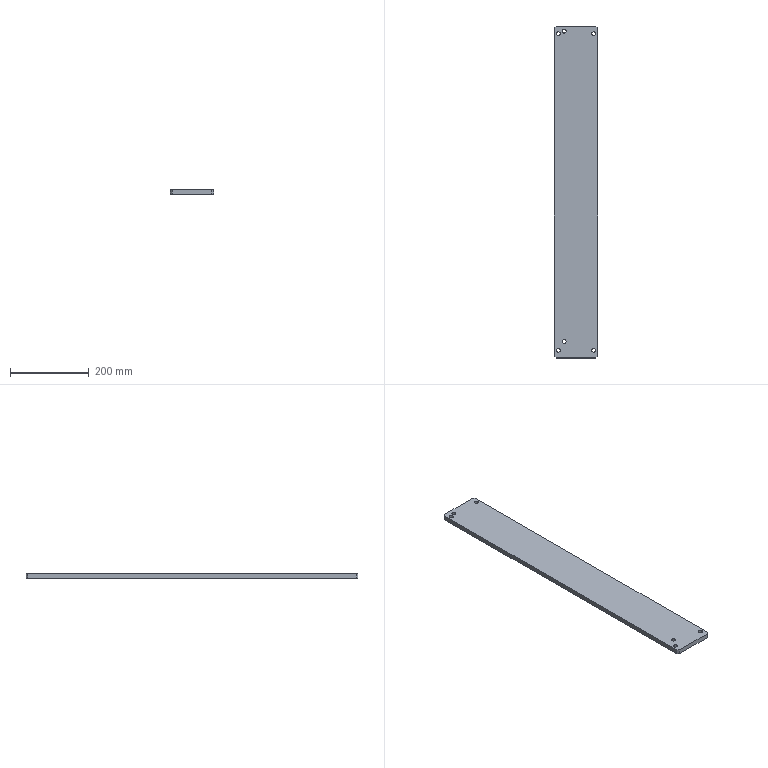Part | STEP file | [24] | 1 solid | 22 faces | box 110 x 844 x 12 mm | volume 1107825 mm3 | cylinder 12 | plane 10 | commonest cylinder face diameters 10 x12
STEP:
#1=CARTESIAN_POINT('',(20.,-727.,0.));
#2=VERTEX_POINT('',#1);
#3=CARTESIAN_POINT('',(30.,-727.,0.));
#4=VERTEX_POINT('',#3);
#5=CARTESIAN_POINT('',(25.,-727.,0.));
#6=DIRECTION('',(0.,0.,1.));
#7=DIRECTION('',(1.,0.,0.));
#8=AXIS2_PLACEMENT_3D('',#5,#6,#7);
#9=CIRCLE('',#8,5.);
#10=EDGE_CURVE('',#2,#4,#9,.T.);
#11=ORIENTED_EDGE('',*,*,#10,.F.);
#12=CARTESIAN_POINT('',(20.,-727.,12.));
#13=VERTEX_POINT('',#12);
#14=CARTESIAN_POINT('',(20.,-727.,0.));
#15=DIRECTION('',(0.,0.,1.));
#16=VECTOR('',#15,1000.);
#17=LINE('',#14,#16);
#18=EDGE_CURVE('',#2,#13,#17,.T.);
#19=ORIENTED_EDGE('',*,*,#18,.T.);
#20=CARTESIAN_POINT('',(30.,-727.,12.));
#21=VERTEX_POINT('',#20);
#22=CARTESIAN_POINT('',(25.,-727.,12.));
#23=DIRECTION('',(0.,0.,-1.));
#24=DIRECTION('',(-1.,0.,0.));
#25=AXIS2_PLACEMENT_3D('',#22,#23,#24);
#26=CIRCLE('',#25,5.);
#27=EDGE_CURVE('',#21,#13,#26,.T.);
#28=ORIENTED_EDGE('',*,*,#27,.F.);
#29=CARTESIAN_POINT('',(30.,-727.,0.));
#30=DIRECTION('',(0.,0.,1.));
#31=VECTOR('',#30,1000.);
#32=LINE('',#29,#31);
#33=EDGE_CURVE('',#4,#21,#32,.T.);
#34=ORIENTED_EDGE('',*,*,#33,.F.);
#35=EDGE_LOOP('',(#11,#19,#28,#34));
#36=FACE_OUTER_BOUND('',#35,.T.);
#37=CARTESIAN_POINT('',(25.,-727.,0.));
#38=DIRECTION('',(0.,0.,1.));
#39=DIRECTION('',(1.,0.,0.));
#40=AXIS2_PLACEMENT_3D('',#37,#38,#39);
#41=CYLINDRICAL_SURFACE('',#40,5.);
#42=ADVANCED_FACE('',(#36),#41,.F.);
#43=CARTESIAN_POINT('',(5.,-749.5,0.));
#44=VERTEX_POINT('',#43);
#45=CARTESIAN_POINT('',(15.,-749.5,0.));
#46=VERTEX_POINT('',#45);
#47=CARTESIAN_POINT('',(10.,-749.5,0.));
#48=DIRECTION('',(0.,0.,1.));
#49=DIRECTION('',(1.,0.,0.));
#50=AXIS2_PLACEMENT_3D('',#47,#48,#49);
#51=CIRCLE('',#50,5.);
#52=EDGE_CURVE('',#44,#46,#51,.T.);
#53=ORIENTED_EDGE('',*,*,#52,.F.);
#54=CARTESIAN_POINT('',(5.,-749.5,12.));
#55=VERTEX_POINT('',#54);
#56=CARTESIAN_POINT('',(5.,-749.5,0.));
#57=DIRECTION('',(0.,0.,1.));
#58=VECTOR('',#57,1000.);
#59=LINE('',#56,#58);
#60=EDGE_CURVE('',#44,#55,#59,.T.);
#61=ORIENTED_EDGE('',*,*,#60,.T.);
#62=CARTESIAN_POINT('',(15.,-749.5,12.));
#63=VERTEX_POINT('',#62);
#64=CARTESIAN_POINT('',(10.,-749.5,12.));
#65=DIRECTION('',(0.,0.,-1.));
#66=DIRECTION('',(-1.,0.,0.));
#67=AXIS2_PLACEMENT_3D('',#64,#65,#66);
#68=CIRCLE('',#67,5.);
#69=EDGE_CURVE('',#63,#55,#68,.T.);
#70=ORIENTED_EDGE('',*,*,#69,.F.);
#71=CARTESIAN_POINT('',(15.,-749.5,0.));
#72=DIRECTION('',(0.,0.,1.));
#73=VECTOR('',#72,1000.);
#74=LINE('',#71,#73);
#75=EDGE_CURVE('',#46,#63,#74,.T.);
#76=ORIENTED_EDGE('',*,*,#75,.F.);
#77=EDGE_LOOP('',(#53,#61,#70,#76));
#78=FACE_OUTER_BOUND('',#77,.T.);
#79=CARTESIAN_POINT('',(10.,-749.5,0.));
#80=DIRECTION('',(0.,0.,1.));
#81=DIRECTION('',(1.,0.,0.));
#82=AXIS2_PLACEMENT_3D('',#79,#80,#81);
#83=CYLINDRICAL_SURFACE('',#82,5.);
#84=ADVANCED_FACE('',(#78),#83,.F.);
#85=CARTESIAN_POINT('',(95.,-749.5,0.));
#86=VERTEX_POINT('',#85);
#87=CARTESIAN_POINT('',(105.,-749.5,0.));
#88=VERTEX_POINT('',#87);
#89=CARTESIAN_POINT('',(100.,-749.5,0.));
#90=DIRECTION('',(0.,0.,1.));
#91=DIRECTION('',(1.,0.,0.));
#92=AXIS2_PLACEMENT_3D('',#89,#90,#91);
#93=CIRCLE('',#92,5.);
#94=EDGE_CURVE('',#86,#88,#93,.T.);
#95=ORIENTED_EDGE('',*,*,#94,.F.);
#96=CARTESIAN_POINT('',(95.,-749.5,12.));
#97=VERTEX_POINT('',#96);
#98=CARTESIAN_POINT('',(95.,-749.5,0.));
#99=DIRECTION('',(0.,0.,1.));
#100=VECTOR('',#99,1000.);
#101=LINE('',#98,#100);
#102=EDGE_CURVE('',#86,#97,#101,.T.);
#103=ORIENTED_EDGE('',*,*,#102,.T.);
#104=CARTESIAN_POINT('',(105.,-749.5,12.));
#105=VERTEX_POINT('',#104);
#106=CARTESIAN_POINT('',(100.,-749.5,12.));
#107=DIRECTION('',(0.,0.,-1.));
#108=DIRECTION('',(-1.,0.,0.));
#109=AXIS2_PLACEMENT_3D('',#106,#107,#108);
#110=CIRCLE('',#109,5.);
#111=EDGE_CURVE('',#105,#97,#110,.T.);
#112=ORIENTED_EDGE('',*,*,#111,.F.);
#113=CARTESIAN_POINT('',(105.,-749.5,0.));
#114=DIRECTION('',(0.,0.,1.));
#115=VECTOR('',#114,1000.);
#116=LINE('',#113,#115);
#117=EDGE_CURVE('',#88,#105,#116,.T.);
#118=ORIENTED_EDGE('',*,*,#117,.F.);
#119=EDGE_LOOP('',(#95,#103,#112,#118));
#120=FACE_OUTER_BOUND('',#119,.T.);
#121=CARTESIAN_POINT('',(100.,-749.5,0.));
#122=DIRECTION('',(0.,0.,1.));
#123=DIRECTION('',(1.,0.,0.));
#124=AXIS2_PLACEMENT_3D('',#121,#122,#123);
#125=CYLINDRICAL_SURFACE('',#124,5.);
#126=ADVANCED_FACE('',(#120),#125,.F.);
#127=CARTESIAN_POINT('',(20.,62.,0.));
#128=VERTEX_POINT('',#127);
#129=CARTESIAN_POINT('',(30.,62.,0.));
#130=VERTEX_POINT('',#129);
#131=CARTESIAN_POINT('',(25.,62.,0.));
#132=DIRECTION('',(0.,0.,1.));
#133=DIRECTION('',(1.,0.,0.));
#134=AXIS2_PLACEMENT_3D('',#131,#132,#133);
#135=CIRCLE('',#134,5.);
#136=EDGE_CURVE('',#128,#130,#135,.T.);
#137=ORIENTED_EDGE('',*,*,#136,.F.);
#138=CARTESIAN_POINT('',(20.,62.,12.));
#139=VERTEX_POINT('',#138);
#140=CARTESIAN_POINT('',(20.,62.,0.));
#141=DIRECTION('',(0.,0.,1.));
#142=VECTOR('',#141,1000.);
#143=LINE('',#140,#142);
#144=EDGE_CURVE('',#128,#139,#143,.T.);
#145=ORIENTED_EDGE('',*,*,#144,.T.);
#146=CARTESIAN_POINT('',(30.,62.,12.));
#147=VERTEX_POINT('',#146);
#148=CARTESIAN_POINT('',(25.,62.,12.));
#149=DIRECTION('',(0.,0.,-1.));
#150=DIRECTION('',(-1.,0.,0.));
#151=AXIS2_PLACEMENT_3D('',#148,#149,#150);
#152=CIRCLE('',#151,5.);
#153=EDGE_CURVE('',#147,#139,#152,.T.);
#154=ORIENTED_EDGE('',*,*,#153,.F.);
#155=CARTESIAN_POINT('',(30.,62.,0.));
#156=DIRECTION('',(0.,0.,1.));
#157=VECTOR('',#156,1000.);
#158=LINE('',#155,#157);
#159=EDGE_CURVE('',#130,#147,#158,.T.);
#160=ORIENTED_EDGE('',*,*,#159,.F.);
#161=EDGE_LOOP('',(#137,#145,#154,#160));
#162=FACE_OUTER_BOUND('',#161,.T.);
#163=CARTESIAN_POINT('',(25.,62.,0.));
#164=DIRECTION('',(0.,0.,1.));
#165=DIRECTION('',(1.,0.,0.));
#166=AXIS2_PLACEMENT_3D('',#163,#164,#165);
#167=CYLINDRICAL_SURFACE('',#166,5.);
#168=ADVANCED_FACE('',(#162),#167,.F.);
#169=CARTESIAN_POINT('',(95.,55.5,0.));
#170=VERTEX_POINT('',#169);
#171=CARTESIAN_POINT('',(105.,55.5,0.));
#172=VERTEX_POINT('',#171);
#173=CARTESIAN_POINT('',(100.,55.5,0.));
#174=DIRECTION('',(0.,0.,1.));
#175=DIRECTION('',(1.,0.,0.));
#176=AXIS2_PLACEMENT_3D('',#173,#174,#175);
#177=CIRCLE('',#176,5.);
#178=EDGE_CURVE('',#170,#172,#177,.T.);
#179=ORIENTED_EDGE('',*,*,#178,.F.);
#180=CARTESIAN_POINT('',(95.,55.5,12.));
#181=VERTEX_POINT('',#180);
#182=CARTESIAN_POINT('',(95.,55.5,0.));
#183=DIRECTION('',(0.,0.,1.));
#184=VECTOR('',#183,1000.);
#185=LINE('',#182,#184);
#186=EDGE_CURVE('',#170,#181,#185,.T.);
#187=ORIENTED_EDGE('',*,*,#186,.T.);
#188=CARTESIAN_POINT('',(105.,55.5,12.));
#189=VERTEX_POINT('',#188);
#190=CARTESIAN_POINT('',(100.,55.5,12.));
#191=DIRECTION('',(0.,0.,-1.));
#192=DIRECTION('',(-1.,0.,0.));
#193=AXIS2_PLACEMENT_3D('',#190,#191,#192);
#194=CIRCLE('',#193,5.);
#195=EDGE_CURVE('',#189,#181,#194,.T.);
#196=ORIENTED_EDGE('',*,*,#195,.F.);
#197=CARTESIAN_POINT('',(105.,55.5,0.));
#198=DIRECTION('',(0.,0.,1.));
#199=VECTOR('',#198,1000.);
#200=LINE('',#197,#199);
#201=EDGE_CURVE('',#172,#189,#200,.T.);
#202=ORIENTED_EDGE('',*,*,#201,.F.);
#203=EDGE_LOOP('',(#179,#187,#196,#202));
#204=FACE_OUTER_BOUND('',#203,.T.);
#205=CARTESIAN_POINT('',(100.,55.5,0.));
#206=DIRECTION('',(0.,0.,1.));
#207=DIRECTION('',(1.,0.,0.));
#208=AXIS2_PLACEMENT_3D('',#205,#206,#207);
#209=CYLINDRICAL_SURFACE('',#208,5.);
#210=ADVANCED_FACE('',(#204),#209,.F.);
#211=CARTESIAN_POINT('',(5.,55.5,0.));
#212=VERTEX_POINT('',#211);
#213=CARTESIAN_POINT('',(15.,55.5,0.));
#214=VERTEX_POINT('',#213);
#215=CARTESIAN_POINT('',(10.,55.5,0.));
#216=DIRECTION('',(0.,0.,1.));
#217=DIRECTION('',(1.,0.,0.));
#218=AXIS2_PLACEMENT_3D('',#215,#216,#217);
#219=CIRCLE('',#218,5.);
#220=EDGE_CURVE('',#212,#214,#219,.T.);
#221=ORIENTED_EDGE('',*,*,#220,.F.);
#222=CARTESIAN_POINT('',(5.,55.5,12.));
#223=VERTEX_POINT('',#222);
#224=CARTESIAN_POINT('',(5.,55.5,0.));
#225=DIRECTION('',(0.,0.,1.));
#226=VECTOR('',#225,1000.);
#227=LINE('',#224,#226);
#228=EDGE_CURVE('',#212,#223,#227,.T.);
#229=ORIENTED_EDGE('',*,*,#228,.T.);
#230=CARTESIAN_POINT('',(15.,55.5,12.));
#231=VERTEX_POINT('',#230);
#232=CARTESIAN_POINT('',(10.,55.5,12.));
#233=DIRECTION('',(0.,0.,-1.));
#234=DIRECTION('',(-1.,0.,0.));
#235=AXIS2_PLACEMENT_3D('',#232,#233,#234);
#236=CIRCLE('',#235,5.);
#237=EDGE_CURVE('',#231,#223,#236,.T.);
#238=ORIENTED_EDGE('',*,*,#237,.F.);
#239=CARTESIAN_POINT('',(15.,55.5,0.));
#240=DIRECTION('',(0.,0.,1.));
#241=VECTOR('',#240,1000.);
#242=LINE('',#239,#241);
#243=EDGE_CURVE('',#214,#231,#242,.T.);
#244=ORIENTED_EDGE('',*,*,#243,.F.);
#245=EDGE_LOOP('',(#221,#229,#238,#244));
#246=FACE_OUTER_BOUND('',#245,.T.);
#247=CARTESIAN_POINT('',(10.,55.5,0.));
#248=DIRECTION('',(0.,0.,1.));
#249=DIRECTION('',(1.,0.,0.));
#250=AXIS2_PLACEMENT_3D('',#247,#248,#249);
#251=CYLINDRICAL_SURFACE('',#250,5.);
#252=ADVANCED_FACE('',(#246),#251,.F.);
#253=CARTESIAN_POINT('',(25.,62.,0.));
#254=DIRECTION('',(0.,0.,1.));
#255=DIRECTION('',(1.,0.,0.));
#256=AXIS2_PLACEMENT_3D('',#253,#254,#255);
#257=CIRCLE('',#256,5.);
#258=EDGE_CURVE('',#130,#128,#257,.T.);
#259=ORIENTED_EDGE('',*,*,#258,.T.);
#260=ORIENTED_EDGE('',*,*,#136,.T.);
#261=EDGE_LOOP('',(#259,#260));
#262=FACE_BOUND('',#261,.T.);
#263=CARTESIAN_POINT('',(100.,55.5,0.));
#264=DIRECTION('',(0.,0.,1.));
#265=DIRECTION('',(1.,0.,0.));
#266=AXIS2_PLACEMENT_3D('',#263,#264,#265);
#267=CIRCLE('',#266,5.);
#268=EDGE_CURVE('',#172,#170,#267,.T.);
#269=ORIENTED_EDGE('',*,*,#268,.T.);
#270=ORIENTED_EDGE('',*,*,#178,.T.);
#271=EDGE_LOOP('',(#269,#270));
#272=FACE_BOUND('',#271,.T.);
#273=CARTESIAN_POINT('',(10.,55.5,0.));
#274=DIRECTION('',(0.,0.,1.));
#275=DIRECTION('',(1.,0.,0.));
#276=AXIS2_PLACEMENT_3D('',#273,#274,#275);
#277=CIRCLE('',#276,5.);
#278=EDGE_CURVE('',#214,#212,#277,.T.);
#279=ORIENTED_EDGE('',*,*,#278,.T.);
#280=ORIENTED_EDGE('',*,*,#220,.T.);
#281=EDGE_LOOP('',(#279,#280));
#282=FACE_BOUND('',#281,.T.);
#283=CARTESIAN_POINT('',(105.,75.,0.));
#284=VERTEX_POINT('',#283);
#285=CARTESIAN_POINT('',(5.,75.,0.));
#286=VERTEX_POINT('',#285);
#287=CARTESIAN_POINT('',(55.,75.,0.));
#288=DIRECTION('',(-1.,0.,0.));
#289=VECTOR('',#288,1000.);
#290=LINE('',#287,#289);
#291=EDGE_CURVE('',#284,#286,#290,.T.);
#292=ORIENTED_EDGE('',*,*,#291,.F.);
#293=CARTESIAN_POINT('',(110.,70.,0.));
#294=VERTEX_POINT('',#293);
#295=CARTESIAN_POINT('',(98.75,81.25,0.));
#296=DIRECTION('',(0.7071,-0.7071,0.));
#297=VECTOR('',#296,1000.);
#298=LINE('',#295,#297);
#299=EDGE_CURVE('',#284,#294,#298,.T.);
#300=ORIENTED_EDGE('',*,*,#299,.T.);
#301=CARTESIAN_POINT('',(110.,-764.,0.));
#302=VERTEX_POINT('',#301);
#303=CARTESIAN_POINT('',(110.,37.5,0.));
#304=DIRECTION('',(0.,1.,0.));
#305=VECTOR('',#304,1000.);
#306=LINE('',#303,#305);
#307=EDGE_CURVE('',#302,#294,#306,.T.);
#308=ORIENTED_EDGE('',*,*,#307,.F.);
#309=CARTESIAN_POINT('',(105.,-769.,0.));
#310=VERTEX_POINT('',#309);
#311=CARTESIAN_POINT('',(272.25,-601.75,0.));
#312=DIRECTION('',(-0.7071,-0.7071,0.));
#313=VECTOR('',#312,1000.);
#314=LINE('',#311,#313);
#315=EDGE_CURVE('',#302,#310,#314,.T.);
#316=ORIENTED_EDGE('',*,*,#315,.T.);
#317=CARTESIAN_POINT('',(5.,-769.,0.));
#318=VERTEX_POINT('',#317);
#319=CARTESIAN_POINT('',(55.,-769.,0.));
#320=DIRECTION('',(1.,0.,0.));
#321=VECTOR('',#320,1000.);
#322=LINE('',#319,#321);
#323=EDGE_CURVE('',#318,#310,#322,.T.);
#324=ORIENTED_EDGE('',*,*,#323,.F.);
#325=CARTESIAN_POINT('',(0.,-764.,0.));
#326=VERTEX_POINT('',#325);
#327=CARTESIAN_POINT('',(-162.25,-601.75,0.));
#328=DIRECTION('',(-0.7071,0.7071,0.));
#329=VECTOR('',#328,1000.);
#330=LINE('',#327,#329);
#331=EDGE_CURVE('',#318,#326,#330,.T.);
#332=ORIENTED_EDGE('',*,*,#331,.T.);
#333=CARTESIAN_POINT('',(0.,70.,0.));
#334=VERTEX_POINT('',#333);
#335=CARTESIAN_POINT('',(0.,37.5,0.));
#336=DIRECTION('',(0.,-1.,0.));
#337=VECTOR('',#336,1000.);
#338=LINE('',#335,#337);
#339=EDGE_CURVE('',#334,#326,#338,.T.);
#340=ORIENTED_EDGE('',*,*,#339,.F.);
#341=CARTESIAN_POINT('',(11.25,81.25,0.));
#342=DIRECTION('',(0.7071,0.7071,0.));
#343=VECTOR('',#342,1000.);
#344=LINE('',#341,#343);
#345=EDGE_CURVE('',#334,#286,#344,.T.);
#346=ORIENTED_EDGE('',*,*,#345,.T.);
#347=EDGE_LOOP('',(#292,#300,#308,#316,#324,#332,#340,#346));
#348=FACE_OUTER_BOUND('',#347,.T.);
#349=CARTESIAN_POINT('',(25.,-727.,0.));
#350=DIRECTION('',(0.,0.,1.));
#351=DIRECTION('',(1.,0.,0.));
#352=AXIS2_PLACEMENT_3D('',#349,#350,#351);
#353=CIRCLE('',#352,5.);
#354=EDGE_CURVE('',#4,#2,#353,.T.);
#355=ORIENTED_EDGE('',*,*,#354,.T.);
#356=ORIENTED_EDGE('',*,*,#10,.T.);
#357=EDGE_LOOP('',(#355,#356));
#358=FACE_BOUND('',#357,.T.);
#359=CARTESIAN_POINT('',(10.,-749.5,0.));
#360=DIRECTION('',(0.,0.,1.));
#361=DIRECTION('',(1.,0.,0.));
#362=AXIS2_PLACEMENT_3D('',#359,#360,#361);
#363=CIRCLE('',#362,5.);
#364=EDGE_CURVE('',#46,#44,#363,.T.);
#365=ORIENTED_EDGE('',*,*,#364,.T.);
#366=ORIENTED_EDGE('',*,*,#52,.T.);
#367=EDGE_LOOP('',(#365,#366));
#368=FACE_BOUND('',#367,.T.);
#369=CARTESIAN_POINT('',(100.,-749.5,0.));
#370=DIRECTION('',(0.,0.,1.));
#371=DIRECTION('',(1.,0.,0.));
#372=AXIS2_PLACEMENT_3D('',#369,#370,#371);
#373=CIRCLE('',#372,5.);
#374=EDGE_CURVE('',#88,#86,#373,.T.);
#375=ORIENTED_EDGE('',*,*,#374,.T.);
#376=ORIENTED_EDGE('',*,*,#94,.T.);
#377=EDGE_LOOP('',(#375,#376));
#378=FACE_BOUND('',#377,.T.);
#379=CARTESIAN_POINT('',(55.,37.5,0.));
#380=DIRECTION('',(0.,0.,-1.));
#381=DIRECTION('',(-1.,0.,0.));
#382=AXIS2_PLACEMENT_3D('',#379,#380,#381);
#383=PLANE('',#382);
#384=ADVANCED_FACE('',(#262,#272,#282,#348,#358,#368,#378),#383,.T.);
#385=ORIENTED_EDGE('',*,*,#307,.T.);
#386=CARTESIAN_POINT('',(110.,70.,12.));
#387=VERTEX_POINT('',#386);
#388=CARTESIAN_POINT('',(110.,70.,12.));
#389=DIRECTION('',(0.,0.,1.));
#390=VECTOR('',#389,1000.);
#391=LINE('',#388,#390);
#392=EDGE_CURVE('',#294,#387,#391,.T.);
#393=ORIENTED_EDGE('',*,*,#392,.T.);
#394=CARTESIAN_POINT('',(110.,-764.,12.));
#395=VERTEX_POINT('',#394);
#396=CARTESIAN_POINT('',(110.,37.5,12.));
#397=DIRECTION('',(0.,-1.,0.));
#398=VECTOR('',#397,1000.);
#399=LINE('',#396,#398);
#400=EDGE_CURVE('',#387,#395,#399,.T.);
#401=ORIENTED_EDGE('',*,*,#400,.T.);
#402=CARTESIAN_POINT('',(110.,-764.,12.));
#403=DIRECTION('',(0.,0.,-1.));
#404=VECTOR('',#403,1000.);
#405=LINE('',#402,#404);
#406=EDGE_CURVE('',#395,#302,#405,.T.);
#407=ORIENTED_EDGE('',*,*,#406,.T.);
#408=EDGE_LOOP('',(#385,#393,#401,#407));
#409=FACE_OUTER_BOUND('',#408,.T.);
#410=CARTESIAN_POINT('',(110.,37.5,12.));
#411=DIRECTION('',(1.,0.,0.));
#412=DIRECTION('',(0.,0.,-1.));
#413=AXIS2_PLACEMENT_3D('',#410,#411,#412);
#414=PLANE('',#413);
#415=ADVANCED_FACE('',(#409),#414,.T.);
#416=CARTESIAN_POINT('',(5.,75.,12.));
#417=VERTEX_POINT('',#416);
#418=CARTESIAN_POINT('',(105.,75.,12.));
#419=VERTEX_POINT('',#418);
#420=CARTESIAN_POINT('',(55.,75.,12.));
#421=DIRECTION('',(1.,0.,0.));
#422=VECTOR('',#421,1000.);
#423=LINE('',#420,#422);
#424=EDGE_CURVE('',#417,#419,#423,.T.);
#425=ORIENTED_EDGE('',*,*,#424,.T.);
#426=CARTESIAN_POINT('',(105.,75.,12.));
#427=DIRECTION('',(0.,0.,-1.));
#428=VECTOR('',#427,1000.);
#429=LINE('',#426,#428);
#430=EDGE_CURVE('',#419,#284,#429,.T.);
#431=ORIENTED_EDGE('',*,*,#430,.T.);
#432=ORIENTED_EDGE('',*,*,#291,.T.);
#433=CARTESIAN_POINT('',(5.,75.,12.));
#434=DIRECTION('',(0.,0.,1.));
#435=VECTOR('',#434,1000.);
#436=LINE('',#433,#435);
#437=EDGE_CURVE('',#286,#417,#436,.T.);
#438=ORIENTED_EDGE('',*,*,#437,.T.);
#439=EDGE_LOOP('',(#425,#431,#432,#438));
#440=FACE_OUTER_BOUND('',#439,.T.);
#441=CARTESIAN_POINT('',(55.,75.,12.));
#442=DIRECTION('',(0.,1.,0.));
#443=DIRECTION('',(0.,0.,-1.));
#444=AXIS2_PLACEMENT_3D('',#441,#442,#443);
#445=PLANE('',#444);
#446=ADVANCED_FACE('',(#440),#445,.T.);
#447=ORIENTED_EDGE('',*,*,#153,.T.);
#448=CARTESIAN_POINT('',(25.,62.,12.));
#449=DIRECTION('',(0.,0.,-1.));
#450=DIRECTION('',(-1.,0.,0.));
#451=AXIS2_PLACEMENT_3D('',#448,#449,#450);
#452=CIRCLE('',#451,5.);
#453=EDGE_CURVE('',#139,#147,#452,.T.);
#454=ORIENTED_EDGE('',*,*,#453,.T.);
#455=EDGE_LOOP('',(#447,#454));
#456=FACE_BOUND('',#455,.T.);
#457=ORIENTED_EDGE('',*,*,#195,.T.);
#458=CARTESIAN_POINT('',(100.,55.5,12.));
#459=DIRECTION('',(0.,0.,-1.));
#460=DIRECTION('',(-1.,0.,0.));
#461=AXIS2_PLACEMENT_3D('',#458,#459,#460);
#462=CIRCLE('',#461,5.);
#463=EDGE_CURVE('',#181,#189,#462,.T.);
#464=ORIENTED_EDGE('',*,*,#463,.T.);
#465=EDGE_LOOP('',(#457,#464));
#466=FACE_BOUND('',#465,.T.);
#467=ORIENTED_EDGE('',*,*,#237,.T.);
#468=CARTESIAN_POINT('',(10.,55.5,12.));
#469=DIRECTION('',(0.,0.,-1.));
#470=DIRECTION('',(-1.,0.,0.));
#471=AXIS2_PLACEMENT_3D('',#468,#469,#470);
#472=CIRCLE('',#471,5.);
#473=EDGE_CURVE('',#223,#231,#472,.T.);
#474=ORIENTED_EDGE('',*,*,#473,.T.);
#475=EDGE_LOOP('',(#467,#474));
#476=FACE_BOUND('',#475,.T.);
#477=ORIENTED_EDGE('',*,*,#400,.F.);
#478=CARTESIAN_POINT('',(98.75,81.25,12.));
#479=DIRECTION('',(-0.7071,0.7071,0.));
#480=VECTOR('',#479,1000.);
#481=LINE('',#478,#480);
#482=EDGE_CURVE('',#387,#419,#481,.T.);
#483=ORIENTED_EDGE('',*,*,#482,.T.);
#484=ORIENTED_EDGE('',*,*,#424,.F.);
#485=CARTESIAN_POINT('',(0.,70.,12.));
#486=VERTEX_POINT('',#485);
#487=CARTESIAN_POINT('',(11.25,81.25,12.));
#488=DIRECTION('',(-0.7071,-0.7071,0.));
#489=VECTOR('',#488,1000.);
#490=LINE('',#487,#489);
#491=EDGE_CURVE('',#417,#486,#490,.T.);
#492=ORIENTED_EDGE('',*,*,#491,.T.);
#493=CARTESIAN_POINT('',(0.,-764.,12.));
#494=VERTEX_POINT('',#493);
#495=CARTESIAN_POINT('',(0.,37.5,12.));
#496=DIRECTION('',(0.,1.,0.));
#497=VECTOR('',#496,1000.);
#498=LINE('',#495,#497);
#499=EDGE_CURVE('',#494,#486,#498,.T.);
#500=ORIENTED_EDGE('',*,*,#499,.F.);
#501=CARTESIAN_POINT('',(5.,-769.,12.));
#502=VERTEX_POINT('',#501);
#503=CARTESIAN_POINT('',(-162.25,-601.75,12.));
#504=DIRECTION('',(0.7071,-0.7071,0.));
#505=VECTOR('',#504,1000.);
#506=LINE('',#503,#505);
#507=EDGE_CURVE('',#494,#502,#506,.T.);
#508=ORIENTED_EDGE('',*,*,#507,.T.);
#509=CARTESIAN_POINT('',(105.,-769.,12.));
#510=VERTEX_POINT('',#509);
#511=CARTESIAN_POINT('',(55.,-769.,12.));
#512=DIRECTION('',(-1.,0.,0.));
#513=VECTOR('',#512,1000.);
#514=LINE('',#511,#513);
#515=EDGE_CURVE('',#510,#502,#514,.T.);
#516=ORIENTED_EDGE('',*,*,#515,.F.);
#517=CARTESIAN_POINT('',(272.25,-601.75,12.));
#518=DIRECTION('',(0.7071,0.7071,0.));
#519=VECTOR('',#518,1000.);
#520=LINE('',#517,#519);
#521=EDGE_CURVE('',#510,#395,#520,.T.);
#522=ORIENTED_EDGE('',*,*,#521,.T.);
#523=EDGE_LOOP('',(#477,#483,#484,#492,#500,#508,#516,#522));
#524=FACE_OUTER_BOUND('',#523,.T.);
#525=ORIENTED_EDGE('',*,*,#27,.T.);
#526=CARTESIAN_POINT('',(25.,-727.,12.));
#527=DIRECTION('',(0.,0.,-1.));
#528=DIRECTION('',(-1.,0.,0.));
#529=AXIS2_PLACEMENT_3D('',#526,#527,#528);
#530=CIRCLE('',#529,5.);
#531=EDGE_CURVE('',#13,#21,#530,.T.);
#532=ORIENTED_EDGE('',*,*,#531,.T.);
#533=EDGE_LOOP('',(#525,#532));
#534=FACE_BOUND('',#533,.T.);
#535=ORIENTED_EDGE('',*,*,#69,.T.);
#536=CARTESIAN_POINT('',(10.,-749.5,12.));
#537=DIRECTION('',(0.,0.,-1.));
#538=DIRECTION('',(-1.,0.,0.));
#539=AXIS2_PLACEMENT_3D('',#536,#537,#538);
#540=CIRCLE('',#539,5.);
#541=EDGE_CURVE('',#55,#63,#540,.T.);
#542=ORIENTED_EDGE('',*,*,#541,.T.);
#543=EDGE_LOOP('',(#535,#542));
#544=FACE_BOUND('',#543,.T.);
#545=ORIENTED_EDGE('',*,*,#111,.T.);
#546=CARTESIAN_POINT('',(100.,-749.5,12.));
#547=DIRECTION('',(0.,0.,-1.));
#548=DIRECTION('',(-1.,0.,0.));
#549=AXIS2_PLACEMENT_3D('',#546,#547,#548);
#550=CIRCLE('',#549,5.);
#551=EDGE_CURVE('',#97,#105,#550,.T.);
#552=ORIENTED_EDGE('',*,*,#551,.T.);
#553=EDGE_LOOP('',(#545,#552));
#554=FACE_BOUND('',#553,.T.);
#555=CARTESIAN_POINT('',(55.,37.5,12.));
#556=DIRECTION('',(0.,0.,1.));
#557=DIRECTION('',(1.,0.,0.));
#558=AXIS2_PLACEMENT_3D('',#555,#556,#557);
#559=PLANE('',#558);
#560=ADVANCED_FACE('',(#456,#466,#476,#524,#534,#544,#554),#559,.T.);
#561=ORIENTED_EDGE('',*,*,#499,.T.);
#562=CARTESIAN_POINT('',(0.,70.,12.));
#563=DIRECTION('',(0.,0.,-1.));
#564=VECTOR('',#563,1000.);
#565=LINE('',#562,#564);
#566=EDGE_CURVE('',#486,#334,#565,.T.);
#567=ORIENTED_EDGE('',*,*,#566,.T.);
#568=ORIENTED_EDGE('',*,*,#339,.T.);
#569=CARTESIAN_POINT('',(0.,-764.,12.));
#570=DIRECTION('',(0.,0.,1.));
#571=VECTOR('',#570,1000.);
#572=LINE('',#569,#571);
#573=EDGE_CURVE('',#326,#494,#572,.T.);
#574=ORIENTED_EDGE('',*,*,#573,.T.);
#575=EDGE_LOOP('',(#561,#567,#568,#574));
#576=FACE_OUTER_BOUND('',#575,.T.);
#577=CARTESIAN_POINT('',(0.,37.5,12.));
#578=DIRECTION('',(-1.,0.,0.));
#579=DIRECTION('',(0.,0.,1.));
#580=AXIS2_PLACEMENT_3D('',#577,#578,#579);
#581=PLANE('',#580);
#582=ADVANCED_FACE('',(#576),#581,.T.);
#583=ORIENTED_EDGE('',*,*,#491,.F.);
#584=ORIENTED_EDGE('',*,*,#437,.F.);
#585=ORIENTED_EDGE('',*,*,#345,.F.);
#586=ORIENTED_EDGE('',*,*,#566,.F.);
#587=EDGE_LOOP('',(#583,#584,#585,#586));
#588=FACE_OUTER_BOUND('',#587,.T.);
#589=CARTESIAN_POINT('',(0.,70.,12.));
#590=DIRECTION('',(0.7071,-0.7071,0.));
#591=DIRECTION('',(0.,0.,-1.));
#592=AXIS2_PLACEMENT_3D('',#589,#590,#591);
#593=PLANE('',#592);
#594=ADVANCED_FACE('',(#588),#593,.F.);
#595=ORIENTED_EDGE('',*,*,#482,.F.);
#596=ORIENTED_EDGE('',*,*,#392,.F.);
#597=ORIENTED_EDGE('',*,*,#299,.F.);
#598=ORIENTED_EDGE('',*,*,#430,.F.);
#599=EDGE_LOOP('',(#595,#596,#597,#598));
#600=FACE_OUTER_BOUND('',#599,.T.);
#601=CARTESIAN_POINT('',(105.,75.,12.));
#602=DIRECTION('',(-0.7071,-0.7071,0.));
#603=DIRECTION('',(0.,0.,-1.));
#604=AXIS2_PLACEMENT_3D('',#601,#602,#603);
#605=PLANE('',#604);
#606=ADVANCED_FACE('',(#600),#605,.F.);
#607=ORIENTED_EDGE('',*,*,#228,.F.);
#608=ORIENTED_EDGE('',*,*,#278,.F.);
#609=ORIENTED_EDGE('',*,*,#243,.T.);
#610=ORIENTED_EDGE('',*,*,#473,.F.);
#611=EDGE_LOOP('',(#607,#608,#609,#610));
#612=FACE_OUTER_BOUND('',#611,.T.);
#613=CARTESIAN_POINT('',(10.,55.5,0.));
#614=DIRECTION('',(0.,0.,1.));
#615=DIRECTION('',(1.,0.,0.));
#616=AXIS2_PLACEMENT_3D('',#613,#614,#615);
#617=CYLINDRICAL_SURFACE('',#616,5.);
#618=ADVANCED_FACE('',(#612),#617,.F.);
#619=ORIENTED_EDGE('',*,*,#186,.F.);
#620=ORIENTED_EDGE('',*,*,#268,.F.);
#621=ORIENTED_EDGE('',*,*,#201,.T.);
#622=ORIENTED_EDGE('',*,*,#463,.F.);
#623=EDGE_LOOP('',(#619,#620,#621,#622));
#624=FACE_OUTER_BOUND('',#623,.T.);
#625=CARTESIAN_POINT('',(100.,55.5,0.));
#626=DIRECTION('',(0.,0.,1.));
#627=DIRECTION('',(1.,0.,0.));
#628=AXIS2_PLACEMENT_3D('',#625,#626,#627);
#629=CYLINDRICAL_SURFACE('',#628,5.);
#630=ADVANCED_FACE('',(#624),#629,.F.);
#631=ORIENTED_EDGE('',*,*,#144,.F.);
#632=ORIENTED_EDGE('',*,*,#258,.F.);
#633=ORIENTED_EDGE('',*,*,#159,.T.);
#634=ORIENTED_EDGE('',*,*,#453,.F.);
#635=EDGE_LOOP('',(#631,#632,#633,#634));
#636=FACE_OUTER_BOUND('',#635,.T.);
#637=CARTESIAN_POINT('',(25.,62.,0.));
#638=DIRECTION('',(0.,0.,1.));
#639=DIRECTION('',(1.,0.,0.));
#640=AXIS2_PLACEMENT_3D('',#637,#638,#639);
#641=CYLINDRICAL_SURFACE('',#640,5.);
#642=ADVANCED_FACE('',(#636),#641,.F.);
#643=ORIENTED_EDGE('',*,*,#323,.T.);
#644=CARTESIAN_POINT('',(105.,-769.,12.));
#645=DIRECTION('',(0.,0.,1.));
#646=VECTOR('',#645,1000.);
#647=LINE('',#644,#646);
#648=EDGE_CURVE('',#310,#510,#647,.T.);
#649=ORIENTED_EDGE('',*,*,#648,.T.);
#650=ORIENTED_EDGE('',*,*,#515,.T.);
#651=CARTESIAN_POINT('',(5.,-769.,12.));
#652=DIRECTION('',(0.,0.,-1.));
#653=VECTOR('',#652,1000.);
#654=LINE('',#651,#653);
#655=EDGE_CURVE('',#502,#318,#654,.T.);
#656=ORIENTED_EDGE('',*,*,#655,.T.);
#657=EDGE_LOOP('',(#643,#649,#650,#656));
#658=FACE_OUTER_BOUND('',#657,.T.);
#659=CARTESIAN_POINT('',(55.,-769.,12.));
#660=DIRECTION('',(0.,-1.,0.));
#661=DIRECTION('',(0.,0.,-1.));
#662=AXIS2_PLACEMENT_3D('',#659,#660,#661);
#663=PLANE('',#662);
#664=ADVANCED_FACE('',(#658),#663,.T.);
#665=ORIENTED_EDGE('',*,*,#521,.F.);
#666=ORIENTED_EDGE('',*,*,#648,.F.);
#667=ORIENTED_EDGE('',*,*,#315,.F.);
#668=ORIENTED_EDGE('',*,*,#406,.F.);
#669=EDGE_LOOP('',(#665,#666,#667,#668));
#670=FACE_OUTER_BOUND('',#669,.T.);
#671=CARTESIAN_POINT('',(110.,-764.,12.));
#672=DIRECTION('',(-0.7071,0.7071,0.));
#673=DIRECTION('',(0.,0.,-1.));
#674=AXIS2_PLACEMENT_3D('',#671,#672,#673);
#675=PLANE('',#674);
#676=ADVANCED_FACE('',(#670),#675,.F.);
#677=ORIENTED_EDGE('',*,*,#507,.F.);
#678=ORIENTED_EDGE('',*,*,#573,.F.);
#679=ORIENTED_EDGE('',*,*,#331,.F.);
#680=ORIENTED_EDGE('',*,*,#655,.F.);
#681=EDGE_LOOP('',(#677,#678,#679,#680));
#682=FACE_OUTER_BOUND('',#681,.T.);
#683=CARTESIAN_POINT('',(5.,-769.,12.));
#684=DIRECTION('',(0.7071,0.7071,0.));
#685=DIRECTION('',(0.,0.,-1.));
#686=AXIS2_PLACEMENT_3D('',#683,#684,#685);
#687=PLANE('',#686);
#688=ADVANCED_FACE('',(#682),#687,.F.);
#689=ORIENTED_EDGE('',*,*,#102,.F.);
#690=ORIENTED_EDGE('',*,*,#374,.F.);
#691=ORIENTED_EDGE('',*,*,#117,.T.);
#692=ORIENTED_EDGE('',*,*,#551,.F.);
#693=EDGE_LOOP('',(#689,#690,#691,#692));
#694=FACE_OUTER_BOUND('',#693,.T.);
#695=CARTESIAN_POINT('',(100.,-749.5,0.));
#696=DIRECTION('',(0.,0.,1.));
#697=DIRECTION('',(1.,0.,0.));
#698=AXIS2_PLACEMENT_3D('',#695,#696,#697);
#699=CYLINDRICAL_SURFACE('',#698,5.);
#700=ADVANCED_FACE('',(#694),#699,.F.);
#701=ORIENTED_EDGE('',*,*,#60,.F.);
#702=ORIENTED_EDGE('',*,*,#364,.F.);
#703=ORIENTED_EDGE('',*,*,#75,.T.);
#704=ORIENTED_EDGE('',*,*,#541,.F.);
#705=EDGE_LOOP('',(#701,#702,#703,#704));
#706=FACE_OUTER_BOUND('',#705,.T.);
#707=CARTESIAN_POINT('',(10.,-749.5,0.));
#708=DIRECTION('',(0.,0.,1.));
#709=DIRECTION('',(1.,0.,0.));
#710=AXIS2_PLACEMENT_3D('',#707,#708,#709);
#711=CYLINDRICAL_SURFACE('',#710,5.);
#712=ADVANCED_FACE('',(#706),#711,.F.);
#713=ORIENTED_EDGE('',*,*,#18,.F.);
#714=ORIENTED_EDGE('',*,*,#354,.F.);
#715=ORIENTED_EDGE('',*,*,#33,.T.);
#716=ORIENTED_EDGE('',*,*,#531,.F.);
#717=EDGE_LOOP('',(#713,#714,#715,#716));
#718=FACE_OUTER_BOUND('',#717,.T.);
#719=CARTESIAN_POINT('',(25.,-727.,0.));
#720=DIRECTION('',(0.,0.,1.));
#721=DIRECTION('',(1.,0.,0.));
#722=AXIS2_PLACEMENT_3D('',#719,#720,#721);
#723=CYLINDRICAL_SURFACE('',#722,5.);
#724=ADVANCED_FACE('',(#718),#723,.F.);
#725=CLOSED_SHELL('',(#42,#84,#126,#168,#210,#252,#384,#415,#446,#560,#582,#594,#606,#618,#630,#642,#664,#676,#688,#700,#712,#724));
#726=MANIFOLD_SOLID_BREP('',#725);
#727=CARTESIAN_POINT('',(0.,0.,0.));
#728=DIRECTION('',(0.,0.,1.));
#729=DIRECTION('',(1.,0.,0.));
#730=AXIS2_PLACEMENT_3D('',#727,#728,#729);
#731=(LENGTH_UNIT()NAMED_UNIT(*)SI_UNIT(.MILLI.,.METRE.));
#732=UNCERTAINTY_MEASURE_WITH_UNIT(LENGTH_MEASURE(0.00001),#731,'','');
#733=(NAMED_UNIT(*)PLANE_ANGLE_UNIT()SI_UNIT($,.RADIAN.));
#734=(NAMED_UNIT(*)SI_UNIT($,.STERADIAN.)SOLID_ANGLE_UNIT());
#735=(GEOMETRIC_REPRESENTATION_CONTEXT(3)GLOBAL_UNCERTAINTY_ASSIGNED_CONTEXT((#732))GLOBAL_UNIT_ASSIGNED_CONTEXT((#731,#733,#734))REPRESENTATION_CONTEXT('',''));
#736=ADVANCED_BREP_SHAPE_REPRESENTATION('',(#726,#730),#735);